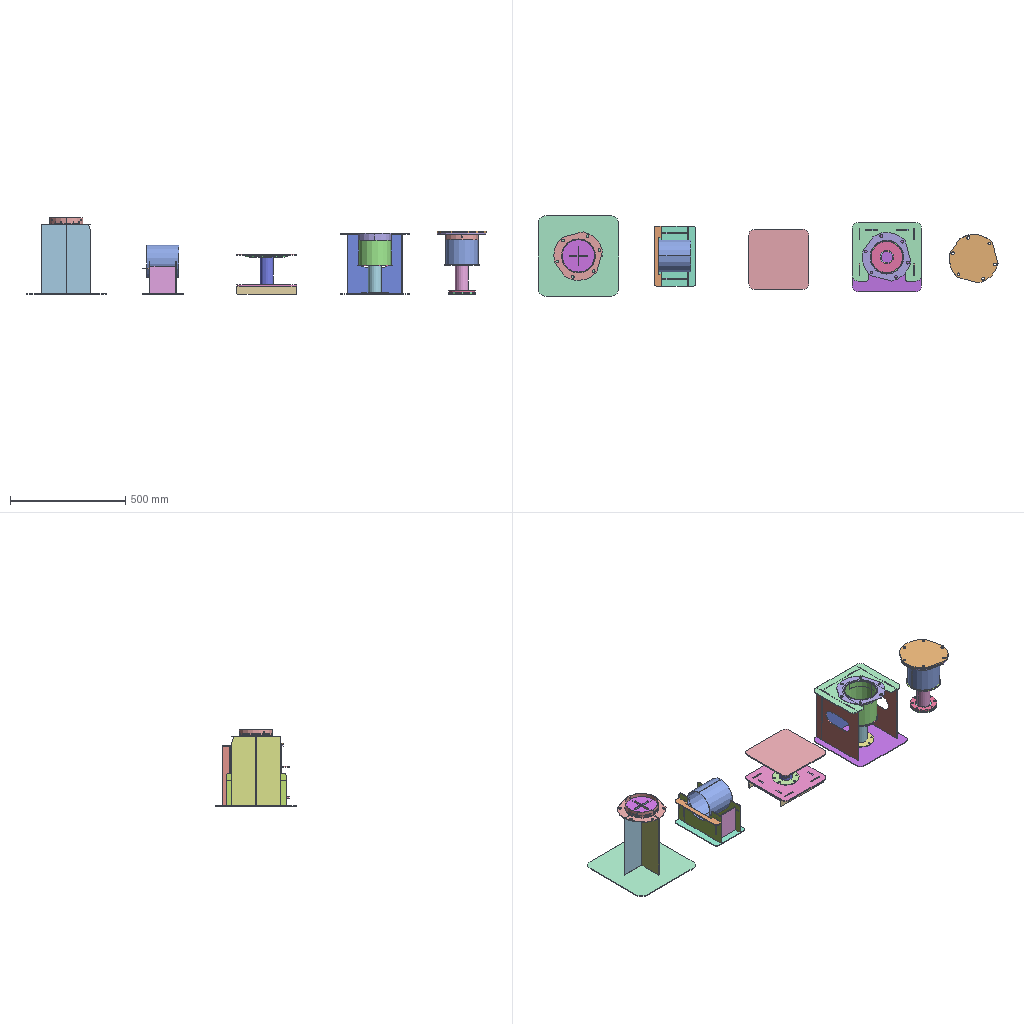Assembly | SolidWorks | 35 different items | 42 placed | box 1994 x 350 x 333 mm
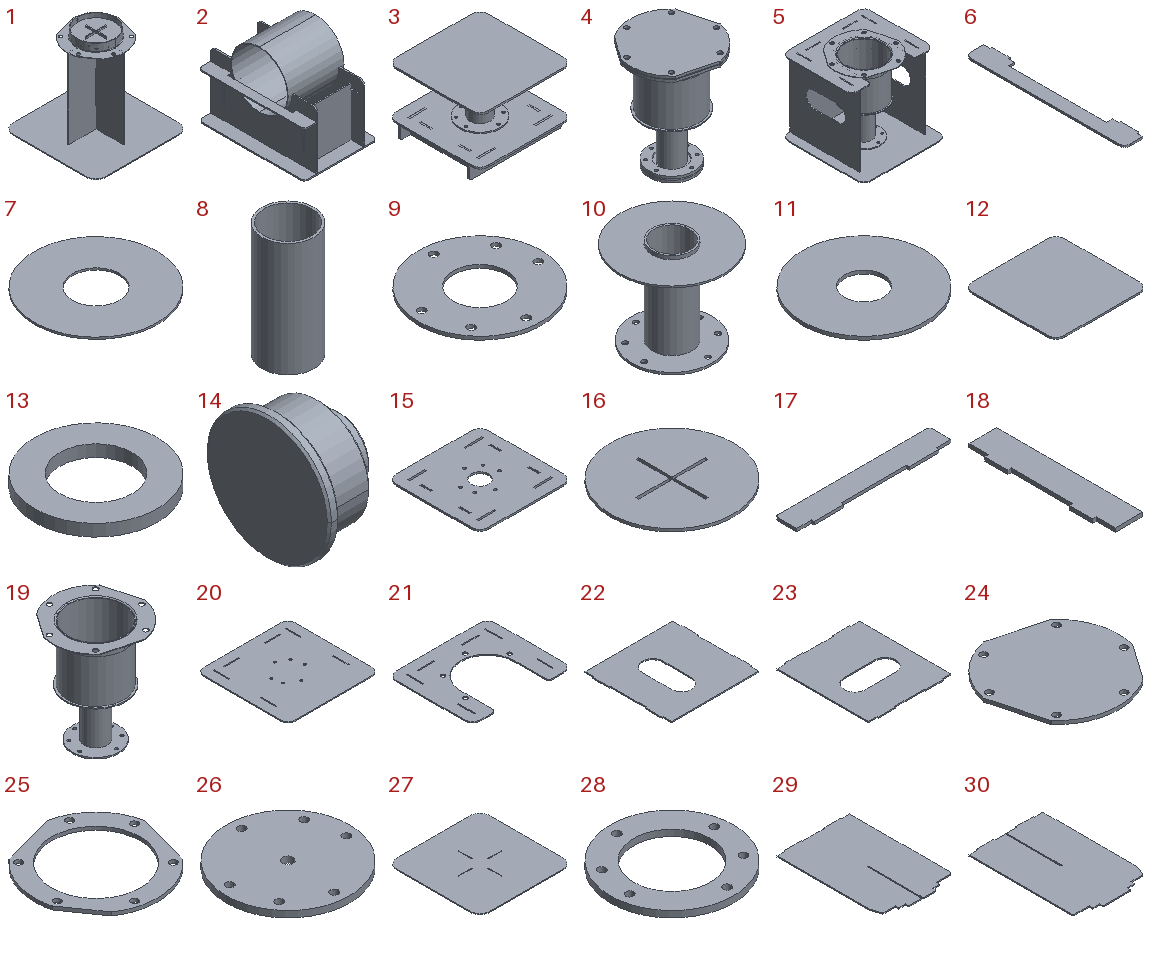Parts list (item | name | quantity | parent item | size | volume | features):
1 | (subassembly) | x1 | - | 350 x 350 x 333.2 mm | 902038 mm3 | -
2 | (subassembly) | x1 | - | 180 x 260 x 213.95 mm | 534069 mm3 | features ReferencePattern 2, LocalLPattern 1, MirrorCompFeat 1
3 | (subassembly) | x1 | - | 260 x 260 x 173.9 mm | 1119008 mm3 | features MirrorCompFeat 2, ReferencePattern 2
4 | (subassembly) | x1 | - | 210.92 x 210.92 x 274.1 mm | 648212 mm3 | features CompositeCurve 1
5 | (subassembly) | x1 | - | 300 x 300 x 265.3 mm | 1237599 mm3 | features MirrorCompFeat 1, ReferencePattern 1
6 | - | x1 | in 2 | 33 x 260 x 3.2 mm | 20279 mm3 | features FlatPattern 1, SMBaseFlange 1, SheetMetal 1
7 | - | x1 | in 4 | 150 x 150 x 2.3 mm | 34755 mm3 | features FlatPattern 1, SMBaseFlange 1, SheetMetal 1
8 | - | x1 | in 4 | 57 x 57 x 124.7 mm | 55410 mm3 | features ExtruThin 1
9 | - | x1 | in 4 | 116 x 116 x 3.2 mm | 26754 mm3 | features FlatPattern 1, SMBaseFlange 1, SheetMetal 1
10 | - | x1 | in 3 | 150 x 150 x 127.9 mm | 116898 mm3 | features BaseBody 5
11 | - | x1 | in 3 | 180 x 180 x 5 mm | 114341 mm3 | features FlatPattern 1, SMBaseFlange 1, SheetMetal 1
12 | - | x1 | in 3 | 260 x 260 x 5 mm | 335317 mm3 | features FlatPattern 1, SMBaseFlange 1, SheetMetal 1
13 | - | x1 | in 3 | 51.7 x 51.7 x 5 mm | 6915 mm3 | features FlatPattern 1, SMBaseFlange 1, SheetMetal 1
14 | - | x1 | in 3 | 35 x 60 x 60 mm | 60166 mm3 | features Chamfer 1, Revolution 1
15 | - | x1 | in 3 | 260 x 260 x 5 mm | 316279 mm3 | features FlatPattern 1, SMBaseFlange 1, SheetMetal 1
16 | - | x1 | in 1 | 141 x 141 x 3.2 mm | 48361 mm3 | features FlatPattern 1, SMBaseFlange 1, SheetMetal 1
17 | - | x2 | in 3 | 260 x 40.5 x 5 mm | 48996 mm3 | features FlatPattern 1, SMBaseFlange 1, SheetMetal 1
18 | - | x2 | in 3 | 40.5 x 190 x 5 mm | 35550 mm3 | features FlatPattern 1, SMBaseFlange 1, SheetMetal 1
19 | - | x1 | in 5 | 210.893 x 210.893 x 262.1 mm | 260766 mm3 | features BaseBody 5
20 | - | x1 | in 5 | 300 x 300 x 3.2 mm | 282429 mm3 | features FlatPattern 1, SMBaseFlange 1, SheetMetal 1
21 | - | x1 | in 5 | 300 x 255 x 3.2 mm | 152496 mm3 | features FlatPattern 1, SMBaseFlange 1, SheetMetal 1
22 | - | x2 | in 5 | 263.3 x 255 x 3.2 mm | 186509 mm3 | features FlatPattern 1, SMBaseFlange 1, SheetMetal 1
23 | - | x1 | in 5 | 233.6 x 263.3 x 3.2 mm | 168889 mm3 | features FlatPattern 1, SMBaseFlange 1, SheetMetal 1
24 | - | x1 | in 4 | 210.92 x 210.92 x 6 mm | 199422 mm3 | features FlatPattern 1, SMBaseFlange 1, SheetMetal 1
25 | - | x1 | in 4 | 210.92 x 210.92 x 6 mm | 89109 mm3 | features FlatPattern 1, SMBaseFlange 1, SheetMetal 1
26 | - | x1 | in 4 | 116 x 116 x 6 mm | 61473 mm3 | features FlatPattern 1, SMBaseFlange 1, SheetMetal 1
27 | - | x1 | in 1 | 350 x 350 x 3.2 mm | 386587 mm3 | features FlatPattern 1, SMBaseFlange 1, SheetMetal 1
28 | - | x1 | in 4 | 116 x 116 x 6 mm | 37515 mm3 | features FlatPattern 1, SMBaseFlange 1, SheetMetal 1
29 | - | x1 | in 1 | 213 x 323 x 3.2 mm | 209682 mm3 | features FlatPattern 1, SMBaseFlange 1, SheetMetal 1
30 | - | x1 | in 1 | 213 x 323 x 3.2 mm | 209682 mm3 | features FlatPattern 1, SMBaseFlange 1, SheetMetal 1
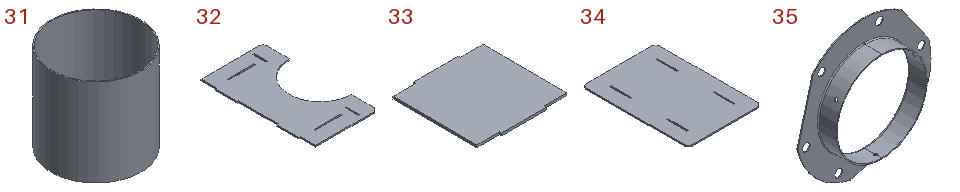31 | - | x2 | in 2, 4 | 140.5 x 140.5 x 137.6 mm | 96049 mm3 | features FlatPattern 1, SMBaseFlange 1, SheetMetal 1
32 | - | x2 | in 2 | 143.5 x 260 x 3.2 mm | 91069 mm3 | features FlatPattern 1, SMBaseFlange 1, SheetMetal 1
33 | - | x2 | in 2 | 120 x 117.8 x 3.2 mm | 44083 mm3 | features FlatPattern 1, SMBaseFlange 1, SheetMetal 1
34 | - | x1 | in 2 | 180 x 260 x 3.2 mm | 147437 mm3 | features FlatPattern 1, SMBaseFlange 1, SheetMetal 1
35 | - | x2 | in 1, 4 | 210.92 x 30 x 210.92 mm | 47725 mm3 | features ICE 3, CirPattern 1, Fillet 1, Revolution 1
Mates (type | each side: item.copy, entity, surface, feature):
In the top assembly
Coincident | 26.1 face plane Base-Flange1 | 20.1 face plane Base-Flange1
Coincident | 18.1 face plane Base-Flange1 | 20.1 face plane Base-Flange1
Coincident | 34.1 face plane Base-Flange1 | 20.1 face plane Base-Flange1
Coincident | 27.1 face plane Base-Flange1 | 34.1 face plane Base-Flange1
In subassembly 4
Coincident | 35.1 face plane Revolve1 | 31.1 face plane BaseBend1
Concentric | 35.1 face cylinder Revolve1 | 31.1 face cylinder BaseBend1
Parallel | 31.1 plane | 4.1 plane
Coincident | 31.1 face plane BaseBend1 | 7.1 face plane Base-Flange1
Concentric | 31.1 face cylinder BaseBend1 | 7.1 face cylinder Base-Flange1
Parallel | 7.1 plane | 4.1 plane
Concentric | 7.1 face cylinder Base-Flange1 | 8.1 face cylinder Extrude-Thin1
DistanceDim | 7.1 face plane Base-Flange1 | 8.1 face plane Extrude-Thin1
Parallel | 8.1 plane | 4.1 plane
Concentric | 8.1 face cylinder Extrude-Thin1 | 9.1 face cylinder Base-Flange1
Coincident | 8.1 face plane Extrude-Thin1 | 9.1 face plane Base-Flange1
Parallel | 9.1 plane | 4.1 plane
InPlace | 35.1 face plane Revolve1 | 24.1 plane
InPlace | 35.1 face plane Revolve1 | 25.1 plane
InPlace | 9.1 face plane Base-Flange1 | 26.2 plane
InPlace | 9.1 face plane Base-Flange1 | 28.1 plane
In subassembly 1
InPlace | 29.1 plane | 1.1 plane
InPlace | 30.1 plane | 1.1 plane
InPlace | 30.1 face plane Base-Flange1 | 16.1 plane
InPlace | 30.1 face plane Base-Flange1 | 27.2 plane
In subassembly 3
InPlace | 10.1 face plane | 15.1 plane
Coincident | 15.1 face plane Base-Flange1 | 14.1 face plane Revolve1
Concentric | 15.1 face cylinder Base-Flange1 | 14.1 face cylinder Revolve1
Parallel | 14.1 plane | 3.1 plane
InPlace | 17.1 plane | 3.1 plane
InPlace | 18.2 plane | 3.1 plane
InPlace | 10.1 face plane | 11.1 plane
InPlace | 11.1 face plane Base-Flange1 | 12.1 plane
InPlace | 14.1 face plane Revolve1 | 13.1 plane
In subassembly 2
InPlace | 32.1 plane | 2.1 plane
InPlace | 33.1 plane | 2.1 plane
InPlace | 32.2 face plane Base-Flange1 | 34.2 plane
InPlace | 6.1 plane | 2.1 plane
In subassembly 5
InPlace | 19.1 face plane | 20.2 plane
InPlace | 19.1 face plane | 21.1 plane
InPlace | 22.1 plane | 5.1 plane
InPlace | 23.1 plane | 5.1 plane